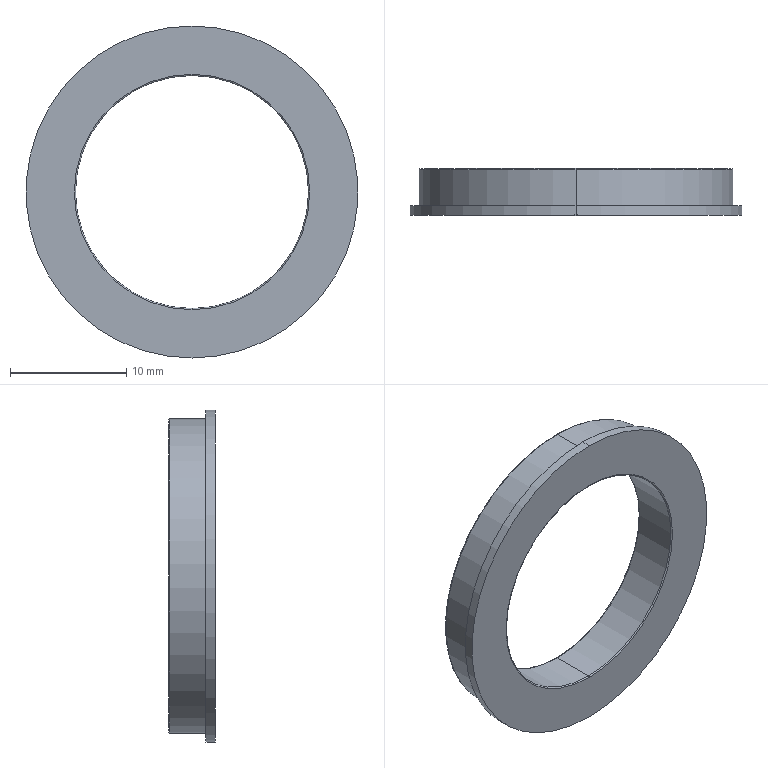Part | SolidWorks | features Extrusion 1, Fillet 1, ICE 1 | 1 solid | 15 faces | box 28.5 x 4 x 28.5 mm | volume 1085 mm3 | torus 6 | cylinder 6 | plane 3 | commonest cylinder face diameters 20 x2 27 x2 28.5 x2
STEP:
#1=CARTESIAN_POINT('',(0.,0.1,-10.));
#2=VERTEX_POINT('',#1);
#3=CARTESIAN_POINT('',(0.,0.1,10.));
#4=VERTEX_POINT('',#3);
#5=CARTESIAN_POINT('',(0.,0.1,0.));
#6=DIRECTION('',(0.,-1.,0.));
#7=DIRECTION('',(0.,0.,1.));
#8=AXIS2_PLACEMENT_3D('',#5,#6,#7);
#9=CIRCLE('',#8,10.);
#10=EDGE_CURVE('',#2,#4,#9,.T.);
#11=ORIENTED_EDGE('',*,*,#10,.F.);
#12=CARTESIAN_POINT('',(0.,0.,-10.1));
#13=VERTEX_POINT('',#12);
#14=CARTESIAN_POINT('',(0.,0.1,-10.1));
#15=DIRECTION('',(1.,0.,0.));
#16=DIRECTION('',(0.,0.,-1.));
#17=AXIS2_PLACEMENT_3D('',#14,#15,#16);
#18=CIRCLE('',#17,0.1);
#19=EDGE_CURVE('',#2,#13,#18,.T.);
#20=ORIENTED_EDGE('',*,*,#19,.T.);
#21=CARTESIAN_POINT('',(0.,0.,10.1));
#22=VERTEX_POINT('',#21);
#23=CARTESIAN_POINT('',(0.,0.,0.));
#24=DIRECTION('',(0.,1.,0.));
#25=DIRECTION('',(0.,0.,1.));
#26=AXIS2_PLACEMENT_3D('',#23,#24,#25);
#27=CIRCLE('',#26,10.1);
#28=EDGE_CURVE('',#22,#13,#27,.T.);
#29=ORIENTED_EDGE('',*,*,#28,.F.);
#30=CARTESIAN_POINT('',(0.,0.1,10.1));
#31=DIRECTION('',(-1.,0.,0.));
#32=DIRECTION('',(0.,0.,1.));
#33=AXIS2_PLACEMENT_3D('',#30,#31,#32);
#34=CIRCLE('',#33,0.1);
#35=EDGE_CURVE('',#4,#22,#34,.T.);
#36=ORIENTED_EDGE('',*,*,#35,.F.);
#37=EDGE_LOOP('',(#11,#20,#29,#36));
#38=FACE_OUTER_BOUND('',#37,.T.);
#39=CARTESIAN_POINT('',(0.,0.1,0.));
#40=DIRECTION('',(0.,1.,0.));
#41=DIRECTION('',(0.,0.,1.));
#42=AXIS2_PLACEMENT_3D('',#39,#40,#41);
#43=TOROIDAL_SURFACE('',#42,10.1,0.1);
#44=ADVANCED_FACE('',(#38),#43,.T.);
#45=CARTESIAN_POINT('',(0.,3.9,-13.5));
#46=VERTEX_POINT('',#45);
#47=CARTESIAN_POINT('',(0.,3.9,13.5));
#48=VERTEX_POINT('',#47);
#49=CARTESIAN_POINT('',(0.,3.9,0.));
#50=DIRECTION('',(0.,-1.,0.));
#51=DIRECTION('',(0.,0.,1.));
#52=AXIS2_PLACEMENT_3D('',#49,#50,#51);
#53=CIRCLE('',#52,13.5);
#54=EDGE_CURVE('',#46,#48,#53,.T.);
#55=ORIENTED_EDGE('',*,*,#54,.F.);
#56=CARTESIAN_POINT('',(0.,4.,-13.4));
#57=VERTEX_POINT('',#56);
#58=CARTESIAN_POINT('',(0.,3.9,-13.4));
#59=DIRECTION('',(1.,0.,0.));
#60=DIRECTION('',(0.,0.,-1.));
#61=AXIS2_PLACEMENT_3D('',#58,#59,#60);
#62=CIRCLE('',#61,0.1);
#63=EDGE_CURVE('',#46,#57,#62,.T.);
#64=ORIENTED_EDGE('',*,*,#63,.T.);
#65=CARTESIAN_POINT('',(0.,4.,13.4));
#66=VERTEX_POINT('',#65);
#67=CARTESIAN_POINT('',(0.,4.,0.));
#68=DIRECTION('',(0.,1.,0.));
#69=DIRECTION('',(0.,0.,1.));
#70=AXIS2_PLACEMENT_3D('',#67,#68,#69);
#71=CIRCLE('',#70,13.4);
#72=EDGE_CURVE('',#66,#57,#71,.T.);
#73=ORIENTED_EDGE('',*,*,#72,.F.);
#74=CARTESIAN_POINT('',(0.,3.9,13.4));
#75=DIRECTION('',(-1.,0.,0.));
#76=DIRECTION('',(0.,0.,1.));
#77=AXIS2_PLACEMENT_3D('',#74,#75,#76);
#78=CIRCLE('',#77,0.1);
#79=EDGE_CURVE('',#48,#66,#78,.T.);
#80=ORIENTED_EDGE('',*,*,#79,.F.);
#81=EDGE_LOOP('',(#55,#64,#73,#80));
#82=FACE_OUTER_BOUND('',#81,.T.);
#83=CARTESIAN_POINT('',(0.,3.9,0.));
#84=DIRECTION('',(0.,1.,0.));
#85=DIRECTION('',(0.,0.,1.));
#86=AXIS2_PLACEMENT_3D('',#83,#84,#85);
#87=TOROIDAL_SURFACE('',#86,13.4,0.1);
#88=ADVANCED_FACE('',(#82),#87,.T.);
#89=CARTESIAN_POINT('',(0.,4.,-10.1));
#90=VERTEX_POINT('',#89);
#91=CARTESIAN_POINT('',(0.,4.,10.1));
#92=VERTEX_POINT('',#91);
#93=CARTESIAN_POINT('',(0.,4.,0.));
#94=DIRECTION('',(0.,-1.,0.));
#95=DIRECTION('',(0.,0.,1.));
#96=AXIS2_PLACEMENT_3D('',#93,#94,#95);
#97=CIRCLE('',#96,10.1);
#98=EDGE_CURVE('',#90,#92,#97,.T.);
#99=ORIENTED_EDGE('',*,*,#98,.F.);
#100=CARTESIAN_POINT('',(0.,3.9,-10.));
#101=VERTEX_POINT('',#100);
#102=CARTESIAN_POINT('',(0.,3.9,-10.1));
#103=DIRECTION('',(1.,0.,0.));
#104=DIRECTION('',(0.,0.,-1.));
#105=AXIS2_PLACEMENT_3D('',#102,#103,#104);
#106=CIRCLE('',#105,0.1);
#107=EDGE_CURVE('',#90,#101,#106,.T.);
#108=ORIENTED_EDGE('',*,*,#107,.T.);
#109=CARTESIAN_POINT('',(0.,3.9,10.));
#110=VERTEX_POINT('',#109);
#111=CARTESIAN_POINT('',(0.,3.9,0.));
#112=DIRECTION('',(0.,1.,0.));
#113=DIRECTION('',(0.,0.,1.));
#114=AXIS2_PLACEMENT_3D('',#111,#112,#113);
#115=CIRCLE('',#114,10.);
#116=EDGE_CURVE('',#110,#101,#115,.T.);
#117=ORIENTED_EDGE('',*,*,#116,.F.);
#118=CARTESIAN_POINT('',(0.,3.9,10.1));
#119=DIRECTION('',(-1.,0.,0.));
#120=DIRECTION('',(0.,0.,1.));
#121=AXIS2_PLACEMENT_3D('',#118,#119,#120);
#122=CIRCLE('',#121,0.1);
#123=EDGE_CURVE('',#92,#110,#122,.T.);
#124=ORIENTED_EDGE('',*,*,#123,.F.);
#125=EDGE_LOOP('',(#99,#108,#117,#124));
#126=FACE_OUTER_BOUND('',#125,.T.);
#127=CARTESIAN_POINT('',(0.,3.9,0.));
#128=DIRECTION('',(0.,1.,0.));
#129=DIRECTION('',(0.,0.,1.));
#130=AXIS2_PLACEMENT_3D('',#127,#128,#129);
#131=TOROIDAL_SURFACE('',#130,10.1,0.1);
#132=ADVANCED_FACE('',(#126),#131,.T.);
#133=ORIENTED_EDGE('',*,*,#54,.T.);
#134=CARTESIAN_POINT('',(0.,0.8,13.5));
#135=VERTEX_POINT('',#134);
#136=CARTESIAN_POINT('',(0.,4.,13.5));
#137=DIRECTION('',(0.,-1.,0.));
#138=VECTOR('',#137,1000.);
#139=LINE('',#136,#138);
#140=EDGE_CURVE('',#48,#135,#139,.T.);
#141=ORIENTED_EDGE('',*,*,#140,.T.);
#142=CARTESIAN_POINT('',(0.,0.8,-13.5));
#143=VERTEX_POINT('',#142);
#144=CARTESIAN_POINT('',(0.,0.8,0.));
#145=DIRECTION('',(0.,1.,0.));
#146=DIRECTION('',(0.,0.,1.));
#147=AXIS2_PLACEMENT_3D('',#144,#145,#146);
#148=CIRCLE('',#147,13.5);
#149=EDGE_CURVE('',#135,#143,#148,.T.);
#150=ORIENTED_EDGE('',*,*,#149,.T.);
#151=CARTESIAN_POINT('',(0.,4.,-13.5));
#152=DIRECTION('',(0.,-1.,0.));
#153=VECTOR('',#152,1000.);
#154=LINE('',#151,#153);
#155=EDGE_CURVE('',#46,#143,#154,.T.);
#156=ORIENTED_EDGE('',*,*,#155,.F.);
#157=EDGE_LOOP('',(#133,#141,#150,#156));
#158=FACE_OUTER_BOUND('',#157,.T.);
#159=CARTESIAN_POINT('',(0.,4.,0.));
#160=DIRECTION('',(0.,-1.,0.));
#161=DIRECTION('',(0.,0.,-1.));
#162=AXIS2_PLACEMENT_3D('',#159,#160,#161);
#163=CYLINDRICAL_SURFACE('',#162,13.5);
#164=ADVANCED_FACE('',(#158),#163,.T.);
#165=CARTESIAN_POINT('',(0.,3.9,0.));
#166=DIRECTION('',(0.,1.,0.));
#167=DIRECTION('',(0.,0.,1.));
#168=AXIS2_PLACEMENT_3D('',#165,#166,#167);
#169=CIRCLE('',#168,10.);
#170=EDGE_CURVE('',#101,#110,#169,.T.);
#171=ORIENTED_EDGE('',*,*,#170,.T.);
#172=CARTESIAN_POINT('',(0.,0.8,10.));
#173=DIRECTION('',(0.,-1.,0.));
#174=VECTOR('',#173,1000.);
#175=LINE('',#172,#174);
#176=EDGE_CURVE('',#110,#4,#175,.T.);
#177=ORIENTED_EDGE('',*,*,#176,.T.);
#178=CARTESIAN_POINT('',(0.,0.1,0.));
#179=DIRECTION('',(0.,-1.,0.));
#180=DIRECTION('',(0.,0.,1.));
#181=AXIS2_PLACEMENT_3D('',#178,#179,#180);
#182=CIRCLE('',#181,10.);
#183=EDGE_CURVE('',#4,#2,#182,.T.);
#184=ORIENTED_EDGE('',*,*,#183,.T.);
#185=CARTESIAN_POINT('',(0.,0.8,-10.));
#186=DIRECTION('',(0.,-1.,0.));
#187=VECTOR('',#186,1000.);
#188=LINE('',#185,#187);
#189=EDGE_CURVE('',#101,#2,#188,.T.);
#190=ORIENTED_EDGE('',*,*,#189,.F.);
#191=EDGE_LOOP('',(#171,#177,#184,#190));
#192=FACE_OUTER_BOUND('',#191,.T.);
#193=CARTESIAN_POINT('',(0.,0.8,0.));
#194=DIRECTION('',(0.,-1.,0.));
#195=DIRECTION('',(0.,0.,-1.));
#196=AXIS2_PLACEMENT_3D('',#193,#194,#195);
#197=CYLINDRICAL_SURFACE('',#196,10.);
#198=ADVANCED_FACE('',(#192),#197,.F.);
#199=CARTESIAN_POINT('',(0.,0.8,14.25));
#200=VERTEX_POINT('',#199);
#201=CARTESIAN_POINT('',(0.,0.8,-14.25));
#202=VERTEX_POINT('',#201);
#203=CARTESIAN_POINT('',(0.,0.8,0.));
#204=DIRECTION('',(0.,1.,0.));
#205=DIRECTION('',(0.,0.,1.));
#206=AXIS2_PLACEMENT_3D('',#203,#204,#205);
#207=CIRCLE('',#206,14.25);
#208=EDGE_CURVE('',#200,#202,#207,.T.);
#209=ORIENTED_EDGE('',*,*,#208,.F.);
#210=CARTESIAN_POINT('',(0.,0.,14.25));
#211=VERTEX_POINT('',#210);
#212=CARTESIAN_POINT('',(0.,0.8,14.25));
#213=DIRECTION('',(0.,-1.,0.));
#214=VECTOR('',#213,1000.);
#215=LINE('',#212,#214);
#216=EDGE_CURVE('',#200,#211,#215,.T.);
#217=ORIENTED_EDGE('',*,*,#216,.T.);
#218=CARTESIAN_POINT('',(0.,0.,-14.25));
#219=VERTEX_POINT('',#218);
#220=CARTESIAN_POINT('',(0.,0.,0.));
#221=DIRECTION('',(0.,1.,0.));
#222=DIRECTION('',(0.,0.,1.));
#223=AXIS2_PLACEMENT_3D('',#220,#221,#222);
#224=CIRCLE('',#223,14.25);
#225=EDGE_CURVE('',#211,#219,#224,.T.);
#226=ORIENTED_EDGE('',*,*,#225,.T.);
#227=CARTESIAN_POINT('',(0.,0.8,-14.25));
#228=DIRECTION('',(0.,-1.,0.));
#229=VECTOR('',#228,1000.);
#230=LINE('',#227,#229);
#231=EDGE_CURVE('',#202,#219,#230,.T.);
#232=ORIENTED_EDGE('',*,*,#231,.F.);
#233=EDGE_LOOP('',(#209,#217,#226,#232));
#234=FACE_OUTER_BOUND('',#233,.T.);
#235=CARTESIAN_POINT('',(0.,0.8,0.));
#236=DIRECTION('',(0.,-1.,0.));
#237=DIRECTION('',(0.,0.,-1.));
#238=AXIS2_PLACEMENT_3D('',#235,#236,#237);
#239=CYLINDRICAL_SURFACE('',#238,14.25);
#240=ADVANCED_FACE('',(#234),#239,.T.);
#241=CARTESIAN_POINT('',(0.,0.8,0.));
#242=DIRECTION('',(0.,1.,0.));
#243=DIRECTION('',(0.,0.,1.));
#244=AXIS2_PLACEMENT_3D('',#241,#242,#243);
#245=CIRCLE('',#244,13.5);
#246=EDGE_CURVE('',#143,#135,#245,.T.);
#247=ORIENTED_EDGE('',*,*,#246,.F.);
#248=ORIENTED_EDGE('',*,*,#149,.F.);
#249=EDGE_LOOP('',(#247,#248));
#250=FACE_BOUND('',#249,.T.);
#251=CARTESIAN_POINT('',(0.,0.8,0.));
#252=DIRECTION('',(0.,1.,0.));
#253=DIRECTION('',(0.,0.,1.));
#254=AXIS2_PLACEMENT_3D('',#251,#252,#253);
#255=CIRCLE('',#254,14.25);
#256=EDGE_CURVE('',#202,#200,#255,.T.);
#257=ORIENTED_EDGE('',*,*,#256,.T.);
#258=ORIENTED_EDGE('',*,*,#208,.T.);
#259=EDGE_LOOP('',(#257,#258));
#260=FACE_OUTER_BOUND('',#259,.T.);
#261=CARTESIAN_POINT('',(0.,0.8,0.));
#262=DIRECTION('',(0.,1.,0.));
#263=DIRECTION('',(0.,0.,1.));
#264=AXIS2_PLACEMENT_3D('',#261,#262,#263);
#265=PLANE('',#264);
#266=ADVANCED_FACE('',(#250,#260),#265,.T.);
#267=ORIENTED_EDGE('',*,*,#28,.T.);
#268=CARTESIAN_POINT('',(0.,0.,0.));
#269=DIRECTION('',(0.,1.,0.));
#270=DIRECTION('',(0.,0.,1.));
#271=AXIS2_PLACEMENT_3D('',#268,#269,#270);
#272=CIRCLE('',#271,10.1);
#273=EDGE_CURVE('',#13,#22,#272,.T.);
#274=ORIENTED_EDGE('',*,*,#273,.T.);
#275=EDGE_LOOP('',(#267,#274));
#276=FACE_BOUND('',#275,.T.);
#277=CARTESIAN_POINT('',(0.,0.,0.));
#278=DIRECTION('',(0.,1.,0.));
#279=DIRECTION('',(0.,0.,1.));
#280=AXIS2_PLACEMENT_3D('',#277,#278,#279);
#281=CIRCLE('',#280,14.25);
#282=EDGE_CURVE('',#219,#211,#281,.T.);
#283=ORIENTED_EDGE('',*,*,#282,.F.);
#284=ORIENTED_EDGE('',*,*,#225,.F.);
#285=EDGE_LOOP('',(#283,#284));
#286=FACE_OUTER_BOUND('',#285,.T.);
#287=CARTESIAN_POINT('',(0.,0.,0.));
#288=DIRECTION('',(0.,1.,0.));
#289=DIRECTION('',(0.,0.,1.));
#290=AXIS2_PLACEMENT_3D('',#287,#288,#289);
#291=PLANE('',#290);
#292=ADVANCED_FACE('',(#276,#286),#291,.F.);
#293=ORIENTED_EDGE('',*,*,#216,.F.);
#294=ORIENTED_EDGE('',*,*,#256,.F.);
#295=ORIENTED_EDGE('',*,*,#231,.T.);
#296=ORIENTED_EDGE('',*,*,#282,.T.);
#297=EDGE_LOOP('',(#293,#294,#295,#296));
#298=FACE_OUTER_BOUND('',#297,.T.);
#299=CARTESIAN_POINT('',(0.,0.8,0.));
#300=DIRECTION('',(0.,-1.,0.));
#301=DIRECTION('',(0.,0.,-1.));
#302=AXIS2_PLACEMENT_3D('',#299,#300,#301);
#303=CYLINDRICAL_SURFACE('',#302,14.25);
#304=ADVANCED_FACE('',(#298),#303,.T.);
#305=ORIENTED_EDGE('',*,*,#176,.F.);
#306=ORIENTED_EDGE('',*,*,#116,.T.);
#307=ORIENTED_EDGE('',*,*,#189,.T.);
#308=ORIENTED_EDGE('',*,*,#10,.T.);
#309=EDGE_LOOP('',(#305,#306,#307,#308));
#310=FACE_OUTER_BOUND('',#309,.T.);
#311=CARTESIAN_POINT('',(0.,0.8,0.));
#312=DIRECTION('',(0.,-1.,0.));
#313=DIRECTION('',(0.,0.,-1.));
#314=AXIS2_PLACEMENT_3D('',#311,#312,#313);
#315=CYLINDRICAL_SURFACE('',#314,10.);
#316=ADVANCED_FACE('',(#310),#315,.F.);
#317=CARTESIAN_POINT('',(0.,4.,0.));
#318=DIRECTION('',(0.,-1.,0.));
#319=DIRECTION('',(0.,0.,1.));
#320=AXIS2_PLACEMENT_3D('',#317,#318,#319);
#321=CIRCLE('',#320,10.1);
#322=EDGE_CURVE('',#92,#90,#321,.T.);
#323=ORIENTED_EDGE('',*,*,#322,.T.);
#324=ORIENTED_EDGE('',*,*,#98,.T.);
#325=EDGE_LOOP('',(#323,#324));
#326=FACE_BOUND('',#325,.T.);
#327=ORIENTED_EDGE('',*,*,#72,.T.);
#328=CARTESIAN_POINT('',(0.,4.,0.));
#329=DIRECTION('',(0.,1.,0.));
#330=DIRECTION('',(0.,0.,1.));
#331=AXIS2_PLACEMENT_3D('',#328,#329,#330);
#332=CIRCLE('',#331,13.4);
#333=EDGE_CURVE('',#57,#66,#332,.T.);
#334=ORIENTED_EDGE('',*,*,#333,.T.);
#335=EDGE_LOOP('',(#327,#334));
#336=FACE_OUTER_BOUND('',#335,.T.);
#337=CARTESIAN_POINT('',(0.,4.,0.));
#338=DIRECTION('',(0.,1.,0.));
#339=DIRECTION('',(0.,0.,1.));
#340=AXIS2_PLACEMENT_3D('',#337,#338,#339);
#341=PLANE('',#340);
#342=ADVANCED_FACE('',(#326,#336),#341,.T.);
#343=ORIENTED_EDGE('',*,*,#140,.F.);
#344=CARTESIAN_POINT('',(0.,3.9,0.));
#345=DIRECTION('',(0.,-1.,0.));
#346=DIRECTION('',(0.,0.,1.));
#347=AXIS2_PLACEMENT_3D('',#344,#345,#346);
#348=CIRCLE('',#347,13.5);
#349=EDGE_CURVE('',#48,#46,#348,.T.);
#350=ORIENTED_EDGE('',*,*,#349,.T.);
#351=ORIENTED_EDGE('',*,*,#155,.T.);
#352=ORIENTED_EDGE('',*,*,#246,.T.);
#353=EDGE_LOOP('',(#343,#350,#351,#352));
#354=FACE_OUTER_BOUND('',#353,.T.);
#355=CARTESIAN_POINT('',(0.,4.,0.));
#356=DIRECTION('',(0.,-1.,0.));
#357=DIRECTION('',(0.,0.,-1.));
#358=AXIS2_PLACEMENT_3D('',#355,#356,#357);
#359=CYLINDRICAL_SURFACE('',#358,13.5);
#360=ADVANCED_FACE('',(#354),#359,.T.);
#361=ORIENTED_EDGE('',*,*,#107,.F.);
#362=ORIENTED_EDGE('',*,*,#322,.F.);
#363=ORIENTED_EDGE('',*,*,#123,.T.);
#364=ORIENTED_EDGE('',*,*,#170,.F.);
#365=EDGE_LOOP('',(#361,#362,#363,#364));
#366=FACE_OUTER_BOUND('',#365,.T.);
#367=CARTESIAN_POINT('',(0.,3.9,0.));
#368=DIRECTION('',(0.,1.,0.));
#369=DIRECTION('',(0.,0.,1.));
#370=AXIS2_PLACEMENT_3D('',#367,#368,#369);
#371=TOROIDAL_SURFACE('',#370,10.1,0.1);
#372=ADVANCED_FACE('',(#366),#371,.T.);
#373=ORIENTED_EDGE('',*,*,#63,.F.);
#374=ORIENTED_EDGE('',*,*,#349,.F.);
#375=ORIENTED_EDGE('',*,*,#79,.T.);
#376=ORIENTED_EDGE('',*,*,#333,.F.);
#377=EDGE_LOOP('',(#373,#374,#375,#376));
#378=FACE_OUTER_BOUND('',#377,.T.);
#379=CARTESIAN_POINT('',(0.,3.9,0.));
#380=DIRECTION('',(0.,1.,0.));
#381=DIRECTION('',(0.,0.,1.));
#382=AXIS2_PLACEMENT_3D('',#379,#380,#381);
#383=TOROIDAL_SURFACE('',#382,13.4,0.1);
#384=ADVANCED_FACE('',(#378),#383,.T.);
#385=ORIENTED_EDGE('',*,*,#19,.F.);
#386=ORIENTED_EDGE('',*,*,#183,.F.);
#387=ORIENTED_EDGE('',*,*,#35,.T.);
#388=ORIENTED_EDGE('',*,*,#273,.F.);
#389=EDGE_LOOP('',(#385,#386,#387,#388));
#390=FACE_OUTER_BOUND('',#389,.T.);
#391=CARTESIAN_POINT('',(0.,0.1,0.));
#392=DIRECTION('',(0.,1.,0.));
#393=DIRECTION('',(0.,0.,1.));
#394=AXIS2_PLACEMENT_3D('',#391,#392,#393);
#395=TOROIDAL_SURFACE('',#394,10.1,0.1);
#396=ADVANCED_FACE('',(#390),#395,.T.);
#397=CLOSED_SHELL('',(#44,#88,#132,#164,#198,#240,#266,#292,#304,#316,#342,#360,#372,#384,#396));
#398=MANIFOLD_SOLID_BREP('',#397);
#399=CARTESIAN_POINT('',(0.,0.,0.));
#400=DIRECTION('',(0.,0.,1.));
#401=DIRECTION('',(1.,0.,0.));
#402=AXIS2_PLACEMENT_3D('',#399,#400,#401);
#403=(LENGTH_UNIT()NAMED_UNIT(*)SI_UNIT(.MILLI.,.METRE.));
#404=UNCERTAINTY_MEASURE_WITH_UNIT(LENGTH_MEASURE(0.00001),#403,'','');
#405=(NAMED_UNIT(*)PLANE_ANGLE_UNIT()SI_UNIT($,.RADIAN.));
#406=(NAMED_UNIT(*)SI_UNIT($,.STERADIAN.)SOLID_ANGLE_UNIT());
#407=(GEOMETRIC_REPRESENTATION_CONTEXT(3)GLOBAL_UNCERTAINTY_ASSIGNED_CONTEXT((#404))GLOBAL_UNIT_ASSIGNED_CONTEXT((#403,#405,#406))REPRESENTATION_CONTEXT('',''));
#408=ADVANCED_BREP_SHAPE_REPRESENTATION('',(#398,#402),#407);